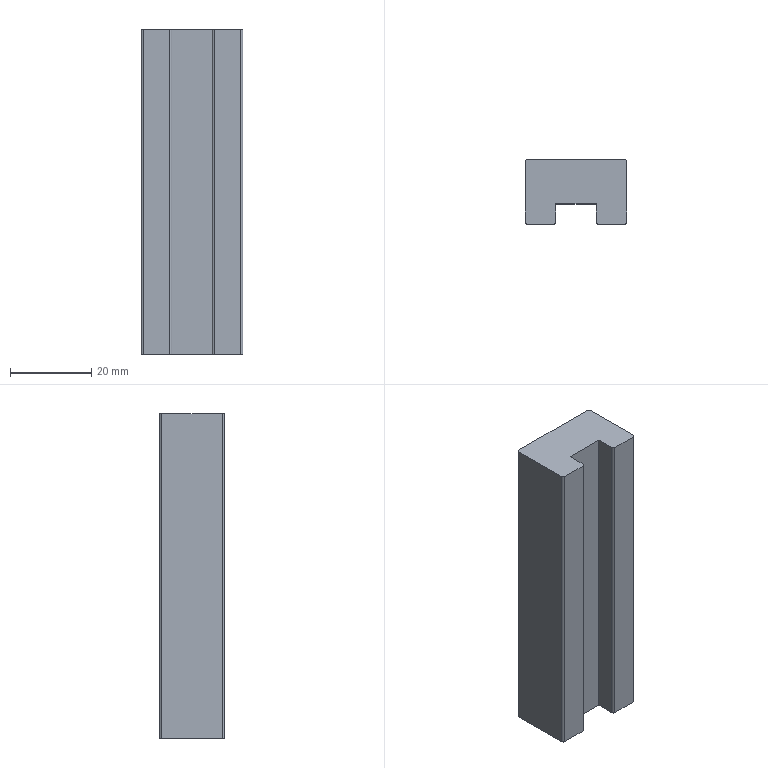Part | STEP file | 1 solid | 19 faces | box 25 x 16 x 80 mm | volume 27687 mm3 | plane 10 | cylinder 7 | cone 2 | commonest cylinder face diameters 1 x6 4.2 x1
STEP:
#1=CARTESIAN_POINT('',(0.,0.,0.));
#2=DIRECTION('',(0.,0.,1.));
#3=DIRECTION('',(1.,0.,0.));
#4=AXIS2_PLACEMENT_3D('',#1,#2,#3);
#5=CARTESIAN_POINT('',(1189.747,499.155,-36.381));
#6=VERTEX_POINT('',#5);
#7=CARTESIAN_POINT('',(1187.247,499.155,-36.381));
#8=DIRECTION('',(0.,0.,1.));
#9=DIRECTION('',(1.,0.,0.));
#10=AXIS2_PLACEMENT_3D('',#7,#8,#9);
#11=CIRCLE('',#10,2.5);
#12=CARTESIAN_POINT('',(1175.247,491.155,-36.381));
#13=DIRECTION('',(0.,0.,1.));
#14=DIRECTION('',(-1.,0.,0.));
#15=AXIS2_PLACEMENT_3D('',#12,#13,#14);
#16=PLANE('',#15);
#17=CARTESIAN_POINT('',(-12.,-8.));
#18=DIRECTION('',(-1.,0.));
#19=AXIS2_PLACEMENT_2D('',#17,#18);
#20=CIRCLE('',#19,2.5);
#21=(GEOMETRIC_REPRESENTATION_CONTEXT(2)PARAMETRIC_REPRESENTATION_CONTEXT()REPRESENTATION_CONTEXT('',''));
#22=DEFINITIONAL_REPRESENTATION('',(#20),#21);
#23=PCURVE('',#16,#22);
#24=CARTESIAN_POINT('',(1187.247,499.155,-36.381));
#25=DIRECTION('',(0.,0.,-1.));
#26=DIRECTION('',(-1.,0.,0.));
#27=AXIS2_PLACEMENT_3D('',#24,#25,#26);
#28=CONICAL_SURFACE('',#27,2.5,0.7854);
#29=CARTESIAN_POINT('',(9.425,0.));
#30=DIRECTION('',(-1.,0.));
#31=VECTOR('',#30,1.);
#32=LINE('',#29,#31);
#33=(GEOMETRIC_REPRESENTATION_CONTEXT(2)PARAMETRIC_REPRESENTATION_CONTEXT()REPRESENTATION_CONTEXT('',''));
#34=DEFINITIONAL_REPRESENTATION('',(#32),#33);
#35=PCURVE('',#28,#34);
#36=SURFACE_CURVE('',#11,(#23,#35),.PCURVE_S1.);
#37=EDGE_CURVE('',#6,#6,#36,.T.);
#38=ORIENTED_EDGE('',*,*,#37,.T.);
#39=EDGE_LOOP('',(#38));
#40=FACE_BOUND('',#39,.T.);
#41=CARTESIAN_POINT('',(1174.747,506.155,-36.381));
#42=VERTEX_POINT('',#41);
#43=CARTESIAN_POINT('',(1174.747,491.155,-36.381));
#44=VERTEX_POINT('',#43);
#45=CARTESIAN_POINT('',(1174.747,506.155,-36.381));
#46=DIRECTION('',(0.,-1.,0.));
#47=VECTOR('',#46,1.);
#48=LINE('',#45,#47);
#49=CARTESIAN_POINT('',(0.5,-15.));
#50=DIRECTION('',(0.,1.));
#51=VECTOR('',#50,1.);
#52=LINE('',#49,#51);
#53=(GEOMETRIC_REPRESENTATION_CONTEXT(2)PARAMETRIC_REPRESENTATION_CONTEXT()REPRESENTATION_CONTEXT('',''));
#54=DEFINITIONAL_REPRESENTATION('',(#52),#53);
#55=PCURVE('',#16,#54);
#56=CARTESIAN_POINT('',(1174.747,506.155,-36.381));
#57=DIRECTION('',(-1.,0.,0.));
#58=DIRECTION('',(0.,0.,-1.));
#59=AXIS2_PLACEMENT_3D('',#56,#57,#58);
#60=PLANE('',#59);
#61=CARTESIAN_POINT('',(0.,0.));
#62=DIRECTION('',(0.,1.));
#63=VECTOR('',#62,1.);
#64=LINE('',#61,#63);
#65=(GEOMETRIC_REPRESENTATION_CONTEXT(2)PARAMETRIC_REPRESENTATION_CONTEXT()REPRESENTATION_CONTEXT('',''));
#66=DEFINITIONAL_REPRESENTATION('',(#64),#65);
#67=PCURVE('',#60,#66);
#68=SURFACE_CURVE('',#48,(#55,#67),.PCURVE_S1.);
#69=EDGE_CURVE('',#42,#44,#68,.T.);
#70=ORIENTED_EDGE('',*,*,#69,.F.);
#71=CARTESIAN_POINT('',(1175.247,506.655,-36.381));
#72=VERTEX_POINT('',#71);
#73=CARTESIAN_POINT('',(1175.247,506.155,-36.381));
#74=DIRECTION('',(0.,0.,1.));
#75=DIRECTION('',(-1.,0.,0.));
#76=AXIS2_PLACEMENT_3D('',#73,#74,#75);
#77=CIRCLE('',#76,0.5);
#78=CARTESIAN_POINT('',(0.,-15.));
#79=DIRECTION('',(1.,0.));
#80=AXIS2_PLACEMENT_2D('',#78,#79);
#81=CIRCLE('',#80,0.5);
#82=(GEOMETRIC_REPRESENTATION_CONTEXT(2)PARAMETRIC_REPRESENTATION_CONTEXT()REPRESENTATION_CONTEXT('',''));
#83=DEFINITIONAL_REPRESENTATION('',(#81),#82);
#84=PCURVE('',#16,#83);
#85=CARTESIAN_POINT('',(1175.247,506.155,-36.381));
#86=DIRECTION('',(0.,0.,1.));
#87=DIRECTION('',(-1.,0.,0.));
#88=AXIS2_PLACEMENT_3D('',#85,#86,#87);
#89=CYLINDRICAL_SURFACE('',#88,0.5);
#90=CARTESIAN_POINT('',(0.,0.));
#91=DIRECTION('',(1.,0.));
#92=VECTOR('',#91,1.);
#93=LINE('',#90,#92);
#94=(GEOMETRIC_REPRESENTATION_CONTEXT(2)PARAMETRIC_REPRESENTATION_CONTEXT()REPRESENTATION_CONTEXT('',''));
#95=DEFINITIONAL_REPRESENTATION('',(#93),#94);
#96=PCURVE('',#89,#95);
#97=SURFACE_CURVE('',#77,(#84,#96),.PCURVE_S1.);
#98=EDGE_CURVE('',#72,#42,#97,.T.);
#99=ORIENTED_EDGE('',*,*,#98,.F.);
#100=CARTESIAN_POINT('',(1199.247,506.655,-36.381));
#101=VERTEX_POINT('',#100);
#102=CARTESIAN_POINT('',(1199.247,506.655,-36.381));
#103=DIRECTION('',(-1.,0.,0.));
#104=VECTOR('',#103,1.);
#105=LINE('',#102,#104);
#106=CARTESIAN_POINT('',(-24.,-15.5));
#107=DIRECTION('',(1.,0.));
#108=VECTOR('',#107,1.);
#109=LINE('',#106,#108);
#110=(GEOMETRIC_REPRESENTATION_CONTEXT(2)PARAMETRIC_REPRESENTATION_CONTEXT()REPRESENTATION_CONTEXT('',''));
#111=DEFINITIONAL_REPRESENTATION('',(#109),#110);
#112=PCURVE('',#16,#111);
#113=CARTESIAN_POINT('',(1199.247,506.655,-36.381));
#114=DIRECTION('',(0.,1.,0.));
#115=DIRECTION('',(0.,0.,1.));
#116=AXIS2_PLACEMENT_3D('',#113,#114,#115);
#117=PLANE('',#116);
#118=CARTESIAN_POINT('',(0.,0.));
#119=DIRECTION('',(0.,-1.));
#120=VECTOR('',#119,1.);
#121=LINE('',#118,#120);
#122=(GEOMETRIC_REPRESENTATION_CONTEXT(2)PARAMETRIC_REPRESENTATION_CONTEXT()REPRESENTATION_CONTEXT('',''));
#123=DEFINITIONAL_REPRESENTATION('',(#121),#122);
#124=PCURVE('',#117,#123);
#125=SURFACE_CURVE('',#105,(#112,#124),.PCURVE_S1.);
#126=EDGE_CURVE('',#101,#72,#125,.T.);
#127=ORIENTED_EDGE('',*,*,#126,.F.);
#128=CARTESIAN_POINT('',(1199.747,506.155,-36.381));
#129=VERTEX_POINT('',#128);
#130=CARTESIAN_POINT('',(1199.247,506.155,-36.381));
#131=DIRECTION('',(0.,0.,1.));
#132=DIRECTION('',(-1.,0.,0.));
#133=AXIS2_PLACEMENT_3D('',#130,#131,#132);
#134=CIRCLE('',#133,0.5);
#135=CARTESIAN_POINT('',(-24.,-15.));
#136=DIRECTION('',(1.,0.));
#137=AXIS2_PLACEMENT_2D('',#135,#136);
#138=CIRCLE('',#137,0.5);
#139=(GEOMETRIC_REPRESENTATION_CONTEXT(2)PARAMETRIC_REPRESENTATION_CONTEXT()REPRESENTATION_CONTEXT('',''));
#140=DEFINITIONAL_REPRESENTATION('',(#138),#139);
#141=PCURVE('',#16,#140);
#142=CARTESIAN_POINT('',(1199.247,506.155,-36.381));
#143=DIRECTION('',(0.,0.,1.));
#144=DIRECTION('',(-1.,0.,0.));
#145=AXIS2_PLACEMENT_3D('',#142,#143,#144);
#146=CYLINDRICAL_SURFACE('',#145,0.5);
#147=CARTESIAN_POINT('',(0.,0.));
#148=DIRECTION('',(1.,0.));
#149=VECTOR('',#148,1.);
#150=LINE('',#147,#149);
#151=(GEOMETRIC_REPRESENTATION_CONTEXT(2)PARAMETRIC_REPRESENTATION_CONTEXT()REPRESENTATION_CONTEXT('',''));
#152=DEFINITIONAL_REPRESENTATION('',(#150),#151);
#153=PCURVE('',#146,#152);
#154=SURFACE_CURVE('',#134,(#141,#153),.PCURVE_S1.);
#155=EDGE_CURVE('',#129,#101,#154,.T.);
#156=ORIENTED_EDGE('',*,*,#155,.F.);
#157=CARTESIAN_POINT('',(1199.747,491.155,-36.381));
#158=VERTEX_POINT('',#157);
#159=CARTESIAN_POINT('',(1199.747,491.155,-36.381));
#160=DIRECTION('',(0.,1.,0.));
#161=VECTOR('',#160,1.);
#162=LINE('',#159,#161);
#163=CARTESIAN_POINT('',(-24.5,0.));
#164=DIRECTION('',(0.,-1.));
#165=VECTOR('',#164,1.);
#166=LINE('',#163,#165);
#167=(GEOMETRIC_REPRESENTATION_CONTEXT(2)PARAMETRIC_REPRESENTATION_CONTEXT()REPRESENTATION_CONTEXT('',''));
#168=DEFINITIONAL_REPRESENTATION('',(#166),#167);
#169=PCURVE('',#16,#168);
#170=CARTESIAN_POINT('',(1199.747,491.155,-36.381));
#171=DIRECTION('',(1.,0.,0.));
#172=DIRECTION('',(0.,0.,1.));
#173=AXIS2_PLACEMENT_3D('',#170,#171,#172);
#174=PLANE('',#173);
#175=CARTESIAN_POINT('',(0.,0.));
#176=DIRECTION('',(0.,-1.));
#177=VECTOR('',#176,1.);
#178=LINE('',#175,#177);
#179=(GEOMETRIC_REPRESENTATION_CONTEXT(2)PARAMETRIC_REPRESENTATION_CONTEXT()REPRESENTATION_CONTEXT('',''));
#180=DEFINITIONAL_REPRESENTATION('',(#178),#179);
#181=PCURVE('',#174,#180);
#182=SURFACE_CURVE('',#162,(#169,#181),.PCURVE_S1.);
#183=EDGE_CURVE('',#158,#129,#182,.T.);
#184=ORIENTED_EDGE('',*,*,#183,.F.);
#185=CARTESIAN_POINT('',(1199.247,490.655,-36.381));
#186=VERTEX_POINT('',#185);
#187=CARTESIAN_POINT('',(1199.247,491.155,-36.381));
#188=DIRECTION('',(0.,0.,1.));
#189=DIRECTION('',(-1.,0.,0.));
#190=AXIS2_PLACEMENT_3D('',#187,#188,#189);
#191=CIRCLE('',#190,0.5);
#192=CARTESIAN_POINT('',(-24.,0.));
#193=DIRECTION('',(1.,0.));
#194=AXIS2_PLACEMENT_2D('',#192,#193);
#195=CIRCLE('',#194,0.5);
#196=(GEOMETRIC_REPRESENTATION_CONTEXT(2)PARAMETRIC_REPRESENTATION_CONTEXT()REPRESENTATION_CONTEXT('',''));
#197=DEFINITIONAL_REPRESENTATION('',(#195),#196);
#198=PCURVE('',#16,#197);
#199=CARTESIAN_POINT('',(1199.247,491.155,-36.381));
#200=DIRECTION('',(0.,0.,1.));
#201=DIRECTION('',(-1.,0.,0.));
#202=AXIS2_PLACEMENT_3D('',#199,#200,#201);
#203=CYLINDRICAL_SURFACE('',#202,0.5);
#204=CARTESIAN_POINT('',(0.,0.));
#205=DIRECTION('',(1.,0.));
#206=VECTOR('',#205,1.);
#207=LINE('',#204,#206);
#208=(GEOMETRIC_REPRESENTATION_CONTEXT(2)PARAMETRIC_REPRESENTATION_CONTEXT()REPRESENTATION_CONTEXT('',''));
#209=DEFINITIONAL_REPRESENTATION('',(#207),#208);
#210=PCURVE('',#203,#209);
#211=SURFACE_CURVE('',#191,(#198,#210),.PCURVE_S1.);
#212=EDGE_CURVE('',#186,#158,#211,.T.);
#213=ORIENTED_EDGE('',*,*,#212,.F.);
#214=CARTESIAN_POINT('',(1192.747,490.655,-36.381));
#215=VERTEX_POINT('',#214);
#216=CARTESIAN_POINT('',(1192.747,490.655,-36.381));
#217=DIRECTION('',(1.,0.,0.));
#218=VECTOR('',#217,1.);
#219=LINE('',#216,#218);
#220=CARTESIAN_POINT('',(-17.5,0.5));
#221=DIRECTION('',(-1.,0.));
#222=VECTOR('',#221,1.);
#223=LINE('',#220,#222);
#224=(GEOMETRIC_REPRESENTATION_CONTEXT(2)PARAMETRIC_REPRESENTATION_CONTEXT()REPRESENTATION_CONTEXT('',''));
#225=DEFINITIONAL_REPRESENTATION('',(#223),#224);
#226=PCURVE('',#16,#225);
#227=CARTESIAN_POINT('',(1192.747,490.655,-36.381));
#228=DIRECTION('',(0.,-1.,0.));
#229=DIRECTION('',(0.,0.,-1.));
#230=AXIS2_PLACEMENT_3D('',#227,#228,#229);
#231=PLANE('',#230);
#232=CARTESIAN_POINT('',(0.,0.));
#233=DIRECTION('',(0.,1.));
#234=VECTOR('',#233,1.);
#235=LINE('',#232,#234);
#236=(GEOMETRIC_REPRESENTATION_CONTEXT(2)PARAMETRIC_REPRESENTATION_CONTEXT()REPRESENTATION_CONTEXT('',''));
#237=DEFINITIONAL_REPRESENTATION('',(#235),#236);
#238=PCURVE('',#231,#237);
#239=SURFACE_CURVE('',#219,(#226,#238),.PCURVE_S1.);
#240=EDGE_CURVE('',#215,#186,#239,.T.);
#241=ORIENTED_EDGE('',*,*,#240,.F.);
#242=CARTESIAN_POINT('',(1192.247,491.155,-36.381));
#243=VERTEX_POINT('',#242);
#244=CARTESIAN_POINT('',(1192.747,491.155,-36.381));
#245=DIRECTION('',(0.,0.,1.));
#246=DIRECTION('',(-1.,0.,0.));
#247=AXIS2_PLACEMENT_3D('',#244,#245,#246);
#248=CIRCLE('',#247,0.5);
#249=CARTESIAN_POINT('',(-17.5,0.));
#250=DIRECTION('',(1.,0.));
#251=AXIS2_PLACEMENT_2D('',#249,#250);
#252=CIRCLE('',#251,0.5);
#253=(GEOMETRIC_REPRESENTATION_CONTEXT(2)PARAMETRIC_REPRESENTATION_CONTEXT()REPRESENTATION_CONTEXT('',''));
#254=DEFINITIONAL_REPRESENTATION('',(#252),#253);
#255=PCURVE('',#16,#254);
#256=CARTESIAN_POINT('',(1192.747,491.155,-36.381));
#257=DIRECTION('',(0.,0.,1.));
#258=DIRECTION('',(-1.,0.,0.));
#259=AXIS2_PLACEMENT_3D('',#256,#257,#258);
#260=CYLINDRICAL_SURFACE('',#259,0.5);
#261=CARTESIAN_POINT('',(0.,0.));
#262=DIRECTION('',(1.,0.));
#263=VECTOR('',#262,1.);
#264=LINE('',#261,#263);
#265=(GEOMETRIC_REPRESENTATION_CONTEXT(2)PARAMETRIC_REPRESENTATION_CONTEXT()REPRESENTATION_CONTEXT('',''));
#266=DEFINITIONAL_REPRESENTATION('',(#264),#265);
#267=PCURVE('',#260,#266);
#268=SURFACE_CURVE('',#248,(#255,#267),.PCURVE_S1.);
#269=EDGE_CURVE('',#243,#215,#268,.T.);
#270=ORIENTED_EDGE('',*,*,#269,.F.);
#271=CARTESIAN_POINT('',(1192.247,495.655,-36.381));
#272=VERTEX_POINT('',#271);
#273=CARTESIAN_POINT('',(1192.247,495.655,-36.381));
#274=DIRECTION('',(0.,-1.,0.));
#275=VECTOR('',#274,1.);
#276=LINE('',#273,#275);
#277=CARTESIAN_POINT('',(-17.,-4.5));
#278=DIRECTION('',(0.,1.));
#279=VECTOR('',#278,1.);
#280=LINE('',#277,#279);
#281=(GEOMETRIC_REPRESENTATION_CONTEXT(2)PARAMETRIC_REPRESENTATION_CONTEXT()REPRESENTATION_CONTEXT('',''));
#282=DEFINITIONAL_REPRESENTATION('',(#280),#281);
#283=PCURVE('',#16,#282);
#284=CARTESIAN_POINT('',(1192.247,495.655,-36.381));
#285=DIRECTION('',(-1.,0.,0.));
#286=DIRECTION('',(0.,0.,-1.));
#287=AXIS2_PLACEMENT_3D('',#284,#285,#286);
#288=PLANE('',#287);
#289=CARTESIAN_POINT('',(0.,0.));
#290=DIRECTION('',(0.,1.));
#291=VECTOR('',#290,1.);
#292=LINE('',#289,#291);
#293=(GEOMETRIC_REPRESENTATION_CONTEXT(2)PARAMETRIC_REPRESENTATION_CONTEXT()REPRESENTATION_CONTEXT('',''));
#294=DEFINITIONAL_REPRESENTATION('',(#292),#293);
#295=PCURVE('',#288,#294);
#296=SURFACE_CURVE('',#276,(#283,#295),.PCURVE_S1.);
#297=EDGE_CURVE('',#272,#243,#296,.T.);
#298=ORIENTED_EDGE('',*,*,#297,.F.);
#299=CARTESIAN_POINT('',(1182.247,495.655,-36.381));
#300=VERTEX_POINT('',#299);
#301=CARTESIAN_POINT('',(1182.247,495.655,-36.381));
#302=DIRECTION('',(1.,0.,0.));
#303=VECTOR('',#302,1.);
#304=LINE('',#301,#303);
#305=CARTESIAN_POINT('',(-7.,-4.5));
#306=DIRECTION('',(-1.,0.));
#307=VECTOR('',#306,1.);
#308=LINE('',#305,#307);
#309=(GEOMETRIC_REPRESENTATION_CONTEXT(2)PARAMETRIC_REPRESENTATION_CONTEXT()REPRESENTATION_CONTEXT('',''));
#310=DEFINITIONAL_REPRESENTATION('',(#308),#309);
#311=PCURVE('',#16,#310);
#312=CARTESIAN_POINT('',(1182.247,495.655,-36.381));
#313=DIRECTION('',(0.,-1.,0.));
#314=DIRECTION('',(0.,0.,-1.));
#315=AXIS2_PLACEMENT_3D('',#312,#313,#314);
#316=PLANE('',#315);
#317=CARTESIAN_POINT('',(0.,0.));
#318=DIRECTION('',(0.,1.));
#319=VECTOR('',#318,1.);
#320=LINE('',#317,#319);
#321=(GEOMETRIC_REPRESENTATION_CONTEXT(2)PARAMETRIC_REPRESENTATION_CONTEXT()REPRESENTATION_CONTEXT('',''));
#322=DEFINITIONAL_REPRESENTATION('',(#320),#321);
#323=PCURVE('',#316,#322);
#324=SURFACE_CURVE('',#304,(#311,#323),.PCURVE_S1.);
#325=EDGE_CURVE('',#300,#272,#324,.T.);
#326=ORIENTED_EDGE('',*,*,#325,.F.);
#327=CARTESIAN_POINT('',(1182.247,491.155,-36.381));
#328=VERTEX_POINT('',#327);
#329=CARTESIAN_POINT('',(1182.247,491.155,-36.381));
#330=DIRECTION('',(0.,1.,0.));
#331=VECTOR('',#330,1.);
#332=LINE('',#329,#331);
#333=CARTESIAN_POINT('',(-7.,0.));
#334=DIRECTION('',(0.,-1.));
#335=VECTOR('',#334,1.);
#336=LINE('',#333,#335);
#337=(GEOMETRIC_REPRESENTATION_CONTEXT(2)PARAMETRIC_REPRESENTATION_CONTEXT()REPRESENTATION_CONTEXT('',''));
#338=DEFINITIONAL_REPRESENTATION('',(#336),#337);
#339=PCURVE('',#16,#338);
#340=CARTESIAN_POINT('',(1182.247,491.155,-36.381));
#341=DIRECTION('',(1.,0.,0.));
#342=DIRECTION('',(0.,0.,1.));
#343=AXIS2_PLACEMENT_3D('',#340,#341,#342);
#344=PLANE('',#343);
#345=CARTESIAN_POINT('',(0.,0.));
#346=DIRECTION('',(0.,-1.));
#347=VECTOR('',#346,1.);
#348=LINE('',#345,#347);
#349=(GEOMETRIC_REPRESENTATION_CONTEXT(2)PARAMETRIC_REPRESENTATION_CONTEXT()REPRESENTATION_CONTEXT('',''));
#350=DEFINITIONAL_REPRESENTATION('',(#348),#349);
#351=PCURVE('',#344,#350);
#352=SURFACE_CURVE('',#332,(#339,#351),.PCURVE_S1.);
#353=EDGE_CURVE('',#328,#300,#352,.T.);
#354=ORIENTED_EDGE('',*,*,#353,.F.);
#355=CARTESIAN_POINT('',(1181.747,490.655,-36.381));
#356=VERTEX_POINT('',#355);
#357=CARTESIAN_POINT('',(1181.747,491.155,-36.381));
#358=DIRECTION('',(0.,0.,1.));
#359=DIRECTION('',(-1.,0.,0.));
#360=AXIS2_PLACEMENT_3D('',#357,#358,#359);
#361=CIRCLE('',#360,0.5);
#362=CARTESIAN_POINT('',(-6.5,0.));
#363=DIRECTION('',(1.,0.));
#364=AXIS2_PLACEMENT_2D('',#362,#363);
#365=CIRCLE('',#364,0.5);
#366=(GEOMETRIC_REPRESENTATION_CONTEXT(2)PARAMETRIC_REPRESENTATION_CONTEXT()REPRESENTATION_CONTEXT('',''));
#367=DEFINITIONAL_REPRESENTATION('',(#365),#366);
#368=PCURVE('',#16,#367);
#369=CARTESIAN_POINT('',(1181.747,491.155,-36.381));
#370=DIRECTION('',(0.,0.,1.));
#371=DIRECTION('',(-1.,0.,0.));
#372=AXIS2_PLACEMENT_3D('',#369,#370,#371);
#373=CYLINDRICAL_SURFACE('',#372,0.5);
#374=CARTESIAN_POINT('',(0.,0.));
#375=DIRECTION('',(1.,0.));
#376=VECTOR('',#375,1.);
#377=LINE('',#374,#376);
#378=(GEOMETRIC_REPRESENTATION_CONTEXT(2)PARAMETRIC_REPRESENTATION_CONTEXT()REPRESENTATION_CONTEXT('',''));
#379=DEFINITIONAL_REPRESENTATION('',(#377),#378);
#380=PCURVE('',#373,#379);
#381=SURFACE_CURVE('',#361,(#368,#380),.PCURVE_S1.);
#382=EDGE_CURVE('',#356,#328,#381,.T.);
#383=ORIENTED_EDGE('',*,*,#382,.F.);
#384=CARTESIAN_POINT('',(1175.247,490.655,-36.381));
#385=VERTEX_POINT('',#384);
#386=CARTESIAN_POINT('',(1175.247,490.655,-36.381));
#387=DIRECTION('',(1.,0.,0.));
#388=VECTOR('',#387,1.);
#389=LINE('',#386,#388);
#390=CARTESIAN_POINT('',(0.,0.5));
#391=DIRECTION('',(-1.,0.));
#392=VECTOR('',#391,1.);
#393=LINE('',#390,#392);
#394=(GEOMETRIC_REPRESENTATION_CONTEXT(2)PARAMETRIC_REPRESENTATION_CONTEXT()REPRESENTATION_CONTEXT('',''));
#395=DEFINITIONAL_REPRESENTATION('',(#393),#394);
#396=PCURVE('',#16,#395);
#397=CARTESIAN_POINT('',(1175.247,490.655,-36.381));
#398=DIRECTION('',(0.,-1.,0.));
#399=DIRECTION('',(0.,0.,-1.));
#400=AXIS2_PLACEMENT_3D('',#397,#398,#399);
#401=PLANE('',#400);
#402=CARTESIAN_POINT('',(0.,0.));
#403=DIRECTION('',(0.,1.));
#404=VECTOR('',#403,1.);
#405=LINE('',#402,#404);
#406=(GEOMETRIC_REPRESENTATION_CONTEXT(2)PARAMETRIC_REPRESENTATION_CONTEXT()REPRESENTATION_CONTEXT('',''));
#407=DEFINITIONAL_REPRESENTATION('',(#405),#406);
#408=PCURVE('',#401,#407);
#409=SURFACE_CURVE('',#389,(#396,#408),.PCURVE_S1.);
#410=EDGE_CURVE('',#385,#356,#409,.T.);
#411=ORIENTED_EDGE('',*,*,#410,.F.);
#412=CARTESIAN_POINT('',(1175.247,491.155,-36.381));
#413=DIRECTION('',(0.,0.,1.));
#414=DIRECTION('',(-1.,0.,0.));
#415=AXIS2_PLACEMENT_3D('',#412,#413,#414);
#416=CIRCLE('',#415,0.5);
#417=CARTESIAN_POINT('',(0.,0.));
#418=DIRECTION('',(1.,0.));
#419=AXIS2_PLACEMENT_2D('',#417,#418);
#420=CIRCLE('',#419,0.5);
#421=(GEOMETRIC_REPRESENTATION_CONTEXT(2)PARAMETRIC_REPRESENTATION_CONTEXT()REPRESENTATION_CONTEXT('',''));
#422=DEFINITIONAL_REPRESENTATION('',(#420),#421);
#423=PCURVE('',#16,#422);
#424=CARTESIAN_POINT('',(1175.247,491.155,-36.381));
#425=DIRECTION('',(0.,0.,1.));
#426=DIRECTION('',(-1.,0.,0.));
#427=AXIS2_PLACEMENT_3D('',#424,#425,#426);
#428=CYLINDRICAL_SURFACE('',#427,0.5);
#429=CARTESIAN_POINT('',(0.,0.));
#430=DIRECTION('',(1.,0.));
#431=VECTOR('',#430,1.);
#432=LINE('',#429,#431);
#433=(GEOMETRIC_REPRESENTATION_CONTEXT(2)PARAMETRIC_REPRESENTATION_CONTEXT()REPRESENTATION_CONTEXT('',''));
#434=DEFINITIONAL_REPRESENTATION('',(#432),#433);
#435=PCURVE('',#428,#434);
#436=SURFACE_CURVE('',#416,(#423,#435),.PCURVE_S1.);
#437=EDGE_CURVE('',#44,#385,#436,.T.);
#438=ORIENTED_EDGE('',*,*,#437,.F.);
#439=EDGE_LOOP('',(#70,#99,#127,#156,#184,#213,#241,#270,#298,#326,#354,#383,#411,#438));
#440=FACE_BOUND('',#439,.T.);
#441=ADVANCED_FACE('',(#40,#440),#16,.F.);
#442=CARTESIAN_POINT('',(1174.747,506.155,43.619));
#443=VERTEX_POINT('',#442);
#444=CARTESIAN_POINT('',(1174.747,491.155,43.619));
#445=VERTEX_POINT('',#444);
#446=CARTESIAN_POINT('',(1174.747,506.155,43.619));
#447=DIRECTION('',(0.,-1.,0.));
#448=VECTOR('',#447,1.);
#449=LINE('',#446,#448);
#450=CARTESIAN_POINT('',(-80.,0.));
#451=DIRECTION('',(0.,1.));
#452=VECTOR('',#451,1.);
#453=LINE('',#450,#452);
#454=(GEOMETRIC_REPRESENTATION_CONTEXT(2)PARAMETRIC_REPRESENTATION_CONTEXT()REPRESENTATION_CONTEXT('',''));
#455=DEFINITIONAL_REPRESENTATION('',(#453),#454);
#456=PCURVE('',#60,#455);
#457=CARTESIAN_POINT('',(1175.247,491.155,43.619));
#458=DIRECTION('',(0.,0.,1.));
#459=DIRECTION('',(-1.,0.,0.));
#460=AXIS2_PLACEMENT_3D('',#457,#458,#459);
#461=PLANE('',#460);
#462=CARTESIAN_POINT('',(0.5,-15.));
#463=DIRECTION('',(0.,1.));
#464=VECTOR('',#463,1.);
#465=LINE('',#462,#464);
#466=(GEOMETRIC_REPRESENTATION_CONTEXT(2)PARAMETRIC_REPRESENTATION_CONTEXT()REPRESENTATION_CONTEXT('',''));
#467=DEFINITIONAL_REPRESENTATION('',(#465),#466);
#468=PCURVE('',#461,#467);
#469=SURFACE_CURVE('',#449,(#456,#468),.PCURVE_S1.);
#470=EDGE_CURVE('',#443,#445,#469,.T.);
#471=ORIENTED_EDGE('',*,*,#470,.F.);
#472=CARTESIAN_POINT('',(1174.747,506.155,-36.381));
#473=DIRECTION('',(0.,0.,1.));
#474=VECTOR('',#473,1.);
#475=LINE('',#472,#474);
#476=CARTESIAN_POINT('',(0.,0.));
#477=DIRECTION('',(-1.,0.));
#478=VECTOR('',#477,1.);
#479=LINE('',#476,#478);
#480=(GEOMETRIC_REPRESENTATION_CONTEXT(2)PARAMETRIC_REPRESENTATION_CONTEXT()REPRESENTATION_CONTEXT('',''));
#481=DEFINITIONAL_REPRESENTATION('',(#479),#480);
#482=PCURVE('',#60,#481);
#483=CARTESIAN_POINT('',(6.283,0.));
#484=DIRECTION('',(0.,1.));
#485=VECTOR('',#484,1.);
#486=LINE('',#483,#485);
#487=(GEOMETRIC_REPRESENTATION_CONTEXT(2)PARAMETRIC_REPRESENTATION_CONTEXT()REPRESENTATION_CONTEXT('',''));
#488=DEFINITIONAL_REPRESENTATION('',(#486),#487);
#489=PCURVE('',#89,#488);
#490=SURFACE_CURVE('',#475,(#482,#489),.PCURVE_S1.);
#491=EDGE_CURVE('',#42,#443,#490,.T.);
#492=ORIENTED_EDGE('',*,*,#491,.F.);
#493=ORIENTED_EDGE('',*,*,#69,.T.);
#494=CARTESIAN_POINT('',(1174.747,491.155,-36.381));
#495=DIRECTION('',(0.,0.,1.));
#496=VECTOR('',#495,1.);
#497=LINE('',#494,#496);
#498=CARTESIAN_POINT('',(0.,15.));
#499=DIRECTION('',(-1.,0.));
#500=VECTOR('',#499,1.);
#501=LINE('',#498,#500);
#502=(GEOMETRIC_REPRESENTATION_CONTEXT(2)PARAMETRIC_REPRESENTATION_CONTEXT()REPRESENTATION_CONTEXT('',''));
#503=DEFINITIONAL_REPRESENTATION('',(#501),#502);
#504=PCURVE('',#60,#503);
#505=CARTESIAN_POINT('',(0.,0.));
#506=DIRECTION('',(0.,1.));
#507=VECTOR('',#506,1.);
#508=LINE('',#505,#507);
#509=(GEOMETRIC_REPRESENTATION_CONTEXT(2)PARAMETRIC_REPRESENTATION_CONTEXT()REPRESENTATION_CONTEXT('',''));
#510=DEFINITIONAL_REPRESENTATION('',(#508),#509);
#511=PCURVE('',#428,#510);
#512=SURFACE_CURVE('',#497,(#504,#511),.PCURVE_S1.);
#513=EDGE_CURVE('',#44,#445,#512,.T.);
#514=ORIENTED_EDGE('',*,*,#513,.T.);
#515=EDGE_LOOP('',(#471,#492,#493,#514));
#516=FACE_BOUND('',#515,.T.);
#517=ADVANCED_FACE('',(#516),#60,.T.);
#518=CARTESIAN_POINT('',(1175.247,490.655,43.619));
#519=VERTEX_POINT('',#518);
#520=CARTESIAN_POINT('',(1175.247,491.155,43.619));
#521=DIRECTION('',(0.,0.,1.));
#522=DIRECTION('',(-1.,0.,0.));
#523=AXIS2_PLACEMENT_3D('',#520,#521,#522);
#524=CIRCLE('',#523,0.5);
#525=CARTESIAN_POINT('',(0.,80.));
#526=DIRECTION('',(1.,0.));
#527=VECTOR('',#526,1.);
#528=LINE('',#525,#527);
#529=(GEOMETRIC_REPRESENTATION_CONTEXT(2)PARAMETRIC_REPRESENTATION_CONTEXT()REPRESENTATION_CONTEXT('',''));
#530=DEFINITIONAL_REPRESENTATION('',(#528),#529);
#531=PCURVE('',#428,#530);
#532=CARTESIAN_POINT('',(0.,0.));
#533=DIRECTION('',(1.,0.));
#534=AXIS2_PLACEMENT_2D('',#532,#533);
#535=CIRCLE('',#534,0.5);
#536=(GEOMETRIC_REPRESENTATION_CONTEXT(2)PARAMETRIC_REPRESENTATION_CONTEXT()REPRESENTATION_CONTEXT('',''));
#537=DEFINITIONAL_REPRESENTATION('',(#535),#536);
#538=PCURVE('',#461,#537);
#539=SURFACE_CURVE('',#524,(#531,#538),.PCURVE_S1.);
#540=EDGE_CURVE('',#445,#519,#539,.T.);
#541=ORIENTED_EDGE('',*,*,#540,.F.);
#542=ORIENTED_EDGE('',*,*,#513,.F.);
#543=ORIENTED_EDGE('',*,*,#437,.T.);
#544=CARTESIAN_POINT('',(1175.247,490.655,-36.381));
#545=DIRECTION('',(0.,0.,1.));
#546=VECTOR('',#545,1.);
#547=LINE('',#544,#546);
#548=CARTESIAN_POINT('',(1.571,0.));
#549=DIRECTION('',(0.,1.));
#550=VECTOR('',#549,1.);
#551=LINE('',#548,#550);
#552=(GEOMETRIC_REPRESENTATION_CONTEXT(2)PARAMETRIC_REPRESENTATION_CONTEXT()REPRESENTATION_CONTEXT('',''));
#553=DEFINITIONAL_REPRESENTATION('',(#551),#552);
#554=PCURVE('',#428,#553);
#555=CARTESIAN_POINT('',(0.,0.));
#556=DIRECTION('',(-1.,0.));
#557=VECTOR('',#556,1.);
#558=LINE('',#555,#557);
#559=(GEOMETRIC_REPRESENTATION_CONTEXT(2)PARAMETRIC_REPRESENTATION_CONTEXT()REPRESENTATION_CONTEXT('',''));
#560=DEFINITIONAL_REPRESENTATION('',(#558),#559);
#561=PCURVE('',#401,#560);
#562=SURFACE_CURVE('',#547,(#554,#561),.PCURVE_S1.);
#563=EDGE_CURVE('',#385,#519,#562,.T.);
#564=ORIENTED_EDGE('',*,*,#563,.T.);
#565=EDGE_LOOP('',(#541,#542,#543,#564));
#566=FACE_BOUND('',#565,.T.);
#567=ADVANCED_FACE('',(#566),#428,.T.);
#568=CARTESIAN_POINT('',(1181.747,490.655,43.619));
#569=VERTEX_POINT('',#568);
#570=CARTESIAN_POINT('',(1175.247,490.655,43.619));
#571=DIRECTION('',(1.,0.,0.));
#572=VECTOR('',#571,1.);
#573=LINE('',#570,#572);
#574=CARTESIAN_POINT('',(-80.,0.));
#575=DIRECTION('',(0.,1.));
#576=VECTOR('',#575,1.);
#577=LINE('',#574,#576);
#578=(GEOMETRIC_REPRESENTATION_CONTEXT(2)PARAMETRIC_REPRESENTATION_CONTEXT()REPRESENTATION_CONTEXT('',''));
#579=DEFINITIONAL_REPRESENTATION('',(#577),#578);
#580=PCURVE('',#401,#579);
#581=CARTESIAN_POINT('',(0.,0.5));
#582=DIRECTION('',(-1.,0.));
#583=VECTOR('',#582,1.);
#584=LINE('',#581,#583);
#585=(GEOMETRIC_REPRESENTATION_CONTEXT(2)PARAMETRIC_REPRESENTATION_CONTEXT()REPRESENTATION_CONTEXT('',''));
#586=DEFINITIONAL_REPRESENTATION('',(#584),#585);
#587=PCURVE('',#461,#586);
#588=SURFACE_CURVE('',#573,(#580,#587),.PCURVE_S1.);
#589=EDGE_CURVE('',#519,#569,#588,.T.);
#590=ORIENTED_EDGE('',*,*,#589,.F.);
#591=ORIENTED_EDGE('',*,*,#563,.F.);
#592=ORIENTED_EDGE('',*,*,#410,.T.);
#593=CARTESIAN_POINT('',(1181.747,490.655,-36.381));
#594=DIRECTION('',(0.,0.,1.));
#595=VECTOR('',#594,1.);
#596=LINE('',#593,#595);
#597=CARTESIAN_POINT('',(0.,6.5));
#598=DIRECTION('',(-1.,0.));
#599=VECTOR('',#598,1.);
#600=LINE('',#597,#599);
#601=(GEOMETRIC_REPRESENTATION_CONTEXT(2)PARAMETRIC_REPRESENTATION_CONTEXT()REPRESENTATION_CONTEXT('',''));
#602=DEFINITIONAL_REPRESENTATION('',(#600),#601);
#603=PCURVE('',#401,#602);
#604=CARTESIAN_POINT('',(1.571,0.));
#605=DIRECTION('',(0.,1.));
#606=VECTOR('',#605,1.);
#607=LINE('',#604,#606);
#608=(GEOMETRIC_REPRESENTATION_CONTEXT(2)PARAMETRIC_REPRESENTATION_CONTEXT()REPRESENTATION_CONTEXT('',''));
#609=DEFINITIONAL_REPRESENTATION('',(#607),#608);
#610=PCURVE('',#373,#609);
#611=SURFACE_CURVE('',#596,(#603,#610),.PCURVE_S1.);
#612=EDGE_CURVE('',#356,#569,#611,.T.);
#613=ORIENTED_EDGE('',*,*,#612,.T.);
#614=EDGE_LOOP('',(#590,#591,#592,#613));
#615=FACE_BOUND('',#614,.T.);
#616=ADVANCED_FACE('',(#615),#401,.T.);
#617=CARTESIAN_POINT('',(1182.247,491.155,43.619));
#618=VERTEX_POINT('',#617);
#619=CARTESIAN_POINT('',(1181.747,491.155,43.619));
#620=DIRECTION('',(0.,0.,1.));
#621=DIRECTION('',(-1.,0.,0.));
#622=AXIS2_PLACEMENT_3D('',#619,#620,#621);
#623=CIRCLE('',#622,0.5);
#624=CARTESIAN_POINT('',(0.,80.));
#625=DIRECTION('',(1.,0.));
#626=VECTOR('',#625,1.);
#627=LINE('',#624,#626);
#628=(GEOMETRIC_REPRESENTATION_CONTEXT(2)PARAMETRIC_REPRESENTATION_CONTEXT()REPRESENTATION_CONTEXT('',''));
#629=DEFINITIONAL_REPRESENTATION('',(#627),#628);
#630=PCURVE('',#373,#629);
#631=CARTESIAN_POINT('',(-6.5,0.));
#632=DIRECTION('',(1.,0.));
#633=AXIS2_PLACEMENT_2D('',#631,#632);
#634=CIRCLE('',#633,0.5);
#635=(GEOMETRIC_REPRESENTATION_CONTEXT(2)PARAMETRIC_REPRESENTATION_CONTEXT()REPRESENTATION_CONTEXT('',''));
#636=DEFINITIONAL_REPRESENTATION('',(#634),#635);
#637=PCURVE('',#461,#636);
#638=SURFACE_CURVE('',#623,(#630,#637),.PCURVE_S1.);
#639=EDGE_CURVE('',#569,#618,#638,.T.);
#640=ORIENTED_EDGE('',*,*,#639,.F.);
#641=ORIENTED_EDGE('',*,*,#612,.F.);
#642=ORIENTED_EDGE('',*,*,#382,.T.);
#643=CARTESIAN_POINT('',(1182.247,491.155,-36.381));
#644=DIRECTION('',(0.,0.,1.));
#645=VECTOR('',#644,1.);
#646=LINE('',#643,#645);
#647=CARTESIAN_POINT('',(3.142,0.));
#648=DIRECTION('',(0.,1.));
#649=VECTOR('',#648,1.);
#650=LINE('',#647,#649);
#651=(GEOMETRIC_REPRESENTATION_CONTEXT(2)PARAMETRIC_REPRESENTATION_CONTEXT()REPRESENTATION_CONTEXT('',''));
#652=DEFINITIONAL_REPRESENTATION('',(#650),#651);
#653=PCURVE('',#373,#652);
#654=CARTESIAN_POINT('',(0.,0.));
#655=DIRECTION('',(1.,0.));
#656=VECTOR('',#655,1.);
#657=LINE('',#654,#656);
#658=(GEOMETRIC_REPRESENTATION_CONTEXT(2)PARAMETRIC_REPRESENTATION_CONTEXT()REPRESENTATION_CONTEXT('',''));
#659=DEFINITIONAL_REPRESENTATION('',(#657),#658);
#660=PCURVE('',#344,#659);
#661=SURFACE_CURVE('',#646,(#653,#660),.PCURVE_S1.);
#662=EDGE_CURVE('',#328,#618,#661,.T.);
#663=ORIENTED_EDGE('',*,*,#662,.T.);
#664=EDGE_LOOP('',(#640,#641,#642,#663));
#665=FACE_BOUND('',#664,.T.);
#666=ADVANCED_FACE('',(#665),#373,.T.);
#667=CARTESIAN_POINT('',(1182.247,495.655,43.619));
#668=VERTEX_POINT('',#667);
#669=CARTESIAN_POINT('',(1182.247,491.155,43.619));
#670=DIRECTION('',(0.,1.,0.));
#671=VECTOR('',#670,1.);
#672=LINE('',#669,#671);
#673=CARTESIAN_POINT('',(80.,0.));
#674=DIRECTION('',(0.,-1.));
#675=VECTOR('',#674,1.);
#676=LINE('',#673,#675);
#677=(GEOMETRIC_REPRESENTATION_CONTEXT(2)PARAMETRIC_REPRESENTATION_CONTEXT()REPRESENTATION_CONTEXT('',''));
#678=DEFINITIONAL_REPRESENTATION('',(#676),#677);
#679=PCURVE('',#344,#678);
#680=CARTESIAN_POINT('',(-7.,0.));
#681=DIRECTION('',(0.,-1.));
#682=VECTOR('',#681,1.);
#683=LINE('',#680,#682);
#684=(GEOMETRIC_REPRESENTATION_CONTEXT(2)PARAMETRIC_REPRESENTATION_CONTEXT()REPRESENTATION_CONTEXT('',''));
#685=DEFINITIONAL_REPRESENTATION('',(#683),#684);
#686=PCURVE('',#461,#685);
#687=SURFACE_CURVE('',#672,(#679,#686),.PCURVE_S1.);
#688=EDGE_CURVE('',#618,#668,#687,.T.);
#689=ORIENTED_EDGE('',*,*,#688,.F.);
#690=ORIENTED_EDGE('',*,*,#662,.F.);
#691=ORIENTED_EDGE('',*,*,#353,.T.);
#692=CARTESIAN_POINT('',(1182.247,495.655,-36.381));
#693=DIRECTION('',(0.,0.,1.));
#694=VECTOR('',#693,1.);
#695=LINE('',#692,#694);
#696=CARTESIAN_POINT('',(0.,-4.5));
#697=DIRECTION('',(1.,0.));
#698=VECTOR('',#697,1.);
#699=LINE('',#696,#698);
#700=(GEOMETRIC_REPRESENTATION_CONTEXT(2)PARAMETRIC_REPRESENTATION_CONTEXT()REPRESENTATION_CONTEXT('',''));
#701=DEFINITIONAL_REPRESENTATION('',(#699),#700);
#702=PCURVE('',#344,#701);
#703=CARTESIAN_POINT('',(0.,0.));
#704=DIRECTION('',(-1.,0.));
#705=VECTOR('',#704,1.);
#706=LINE('',#703,#705);
#707=(GEOMETRIC_REPRESENTATION_CONTEXT(2)PARAMETRIC_REPRESENTATION_CONTEXT()REPRESENTATION_CONTEXT('',''));
#708=DEFINITIONAL_REPRESENTATION('',(#706),#707);
#709=PCURVE('',#316,#708);
#710=SURFACE_CURVE('',#695,(#702,#709),.PCURVE_S1.);
#711=EDGE_CURVE('',#300,#668,#710,.T.);
#712=ORIENTED_EDGE('',*,*,#711,.T.);
#713=EDGE_LOOP('',(#689,#690,#691,#712));
#714=FACE_BOUND('',#713,.T.);
#715=ADVANCED_FACE('',(#714),#344,.T.);
#716=CARTESIAN_POINT('',(1192.247,495.655,43.619));
#717=VERTEX_POINT('',#716);
#718=CARTESIAN_POINT('',(1182.247,495.655,43.619));
#719=DIRECTION('',(1.,0.,0.));
#720=VECTOR('',#719,1.);
#721=LINE('',#718,#720);
#722=CARTESIAN_POINT('',(-80.,0.));
#723=DIRECTION('',(0.,1.));
#724=VECTOR('',#723,1.);
#725=LINE('',#722,#724);
#726=(GEOMETRIC_REPRESENTATION_CONTEXT(2)PARAMETRIC_REPRESENTATION_CONTEXT()REPRESENTATION_CONTEXT('',''));
#727=DEFINITIONAL_REPRESENTATION('',(#725),#726);
#728=PCURVE('',#316,#727);
#729=CARTESIAN_POINT('',(-7.,-4.5));
#730=DIRECTION('',(-1.,0.));
#731=VECTOR('',#730,1.);
#732=LINE('',#729,#731);
#733=(GEOMETRIC_REPRESENTATION_CONTEXT(2)PARAMETRIC_REPRESENTATION_CONTEXT()REPRESENTATION_CONTEXT('',''));
#734=DEFINITIONAL_REPRESENTATION('',(#732),#733);
#735=PCURVE('',#461,#734);
#736=SURFACE_CURVE('',#721,(#728,#735),.PCURVE_S1.);
#737=EDGE_CURVE('',#668,#717,#736,.T.);
#738=ORIENTED_EDGE('',*,*,#737,.F.);
#739=ORIENTED_EDGE('',*,*,#711,.F.);
#740=ORIENTED_EDGE('',*,*,#325,.T.);
#741=CARTESIAN_POINT('',(1192.247,495.655,-36.381));
#742=DIRECTION('',(0.,0.,1.));
#743=VECTOR('',#742,1.);
#744=LINE('',#741,#743);
#745=CARTESIAN_POINT('',(0.,10.));
#746=DIRECTION('',(-1.,0.));
#747=VECTOR('',#746,1.);
#748=LINE('',#745,#747);
#749=(GEOMETRIC_REPRESENTATION_CONTEXT(2)PARAMETRIC_REPRESENTATION_CONTEXT()REPRESENTATION_CONTEXT('',''));
#750=DEFINITIONAL_REPRESENTATION('',(#748),#749);
#751=PCURVE('',#316,#750);
#752=CARTESIAN_POINT('',(0.,0.));
#753=DIRECTION('',(-1.,0.));
#754=VECTOR('',#753,1.);
#755=LINE('',#752,#754);
#756=(GEOMETRIC_REPRESENTATION_CONTEXT(2)PARAMETRIC_REPRESENTATION_CONTEXT()REPRESENTATION_CONTEXT('',''));
#757=DEFINITIONAL_REPRESENTATION('',(#755),#756);
#758=PCURVE('',#288,#757);
#759=SURFACE_CURVE('',#744,(#751,#758),.PCURVE_S1.);
#760=EDGE_CURVE('',#272,#717,#759,.T.);
#761=ORIENTED_EDGE('',*,*,#760,.T.);
#762=EDGE_LOOP('',(#738,#739,#740,#761));
#763=FACE_BOUND('',#762,.T.);
#764=ADVANCED_FACE('',(#763),#316,.T.);
#765=CARTESIAN_POINT('',(1192.247,491.155,43.619));
#766=VERTEX_POINT('',#765);
#767=CARTESIAN_POINT('',(1192.247,495.655,43.619));
#768=DIRECTION('',(0.,-1.,0.));
#769=VECTOR('',#768,1.);
#770=LINE('',#767,#769);
#771=CARTESIAN_POINT('',(-80.,0.));
#772=DIRECTION('',(0.,1.));
#773=VECTOR('',#772,1.);
#774=LINE('',#771,#773);
#775=(GEOMETRIC_REPRESENTATION_CONTEXT(2)PARAMETRIC_REPRESENTATION_CONTEXT()REPRESENTATION_CONTEXT('',''));
#776=DEFINITIONAL_REPRESENTATION('',(#774),#775);
#777=PCURVE('',#288,#776);
#778=CARTESIAN_POINT('',(-17.,-4.5));
#779=DIRECTION('',(0.,1.));
#780=VECTOR('',#779,1.);
#781=LINE('',#778,#780);
#782=(GEOMETRIC_REPRESENTATION_CONTEXT(2)PARAMETRIC_REPRESENTATION_CONTEXT()REPRESENTATION_CONTEXT('',''));
#783=DEFINITIONAL_REPRESENTATION('',(#781),#782);
#784=PCURVE('',#461,#783);
#785=SURFACE_CURVE('',#770,(#777,#784),.PCURVE_S1.);
#786=EDGE_CURVE('',#717,#766,#785,.T.);
#787=ORIENTED_EDGE('',*,*,#786,.F.);
#788=ORIENTED_EDGE('',*,*,#760,.F.);
#789=ORIENTED_EDGE('',*,*,#297,.T.);
#790=CARTESIAN_POINT('',(1192.247,491.155,-36.381));
#791=DIRECTION('',(0.,0.,1.));
#792=VECTOR('',#791,1.);
#793=LINE('',#790,#792);
#794=CARTESIAN_POINT('',(0.,4.5));
#795=DIRECTION('',(-1.,0.));
#796=VECTOR('',#795,1.);
#797=LINE('',#794,#796);
#798=(GEOMETRIC_REPRESENTATION_CONTEXT(2)PARAMETRIC_REPRESENTATION_CONTEXT()REPRESENTATION_CONTEXT('',''));
#799=DEFINITIONAL_REPRESENTATION('',(#797),#798);
#800=PCURVE('',#288,#799);
#801=CARTESIAN_POINT('',(0.,0.));
#802=DIRECTION('',(0.,1.));
#803=VECTOR('',#802,1.);
#804=LINE('',#801,#803);
#805=(GEOMETRIC_REPRESENTATION_CONTEXT(2)PARAMETRIC_REPRESENTATION_CONTEXT()REPRESENTATION_CONTEXT('',''));
#806=DEFINITIONAL_REPRESENTATION('',(#804),#805);
#807=PCURVE('',#260,#806);
#808=SURFACE_CURVE('',#793,(#800,#807),.PCURVE_S1.);
#809=EDGE_CURVE('',#243,#766,#808,.T.);
#810=ORIENTED_EDGE('',*,*,#809,.T.);
#811=EDGE_LOOP('',(#787,#788,#789,#810));
#812=FACE_BOUND('',#811,.T.);
#813=ADVANCED_FACE('',(#812),#288,.T.);
#814=CARTESIAN_POINT('',(1192.747,490.655,43.619));
#815=VERTEX_POINT('',#814);
#816=CARTESIAN_POINT('',(1192.747,491.155,43.619));
#817=DIRECTION('',(0.,0.,1.));
#818=DIRECTION('',(-1.,0.,0.));
#819=AXIS2_PLACEMENT_3D('',#816,#817,#818);
#820=CIRCLE('',#819,0.5);
#821=CARTESIAN_POINT('',(0.,80.));
#822=DIRECTION('',(1.,0.));
#823=VECTOR('',#822,1.);
#824=LINE('',#821,#823);
#825=(GEOMETRIC_REPRESENTATION_CONTEXT(2)PARAMETRIC_REPRESENTATION_CONTEXT()REPRESENTATION_CONTEXT('',''));
#826=DEFINITIONAL_REPRESENTATION('',(#824),#825);
#827=PCURVE('',#260,#826);
#828=CARTESIAN_POINT('',(-17.5,0.));
#829=DIRECTION('',(1.,0.));
#830=AXIS2_PLACEMENT_2D('',#828,#829);
#831=CIRCLE('',#830,0.5);
#832=(GEOMETRIC_REPRESENTATION_CONTEXT(2)PARAMETRIC_REPRESENTATION_CONTEXT()REPRESENTATION_CONTEXT('',''));
#833=DEFINITIONAL_REPRESENTATION('',(#831),#832);
#834=PCURVE('',#461,#833);
#835=SURFACE_CURVE('',#820,(#827,#834),.PCURVE_S1.);
#836=EDGE_CURVE('',#766,#815,#835,.T.);
#837=ORIENTED_EDGE('',*,*,#836,.F.);
#838=ORIENTED_EDGE('',*,*,#809,.F.);
#839=ORIENTED_EDGE('',*,*,#269,.T.);
#840=CARTESIAN_POINT('',(1192.747,490.655,-36.381));
#841=DIRECTION('',(0.,0.,1.));
#842=VECTOR('',#841,1.);
#843=LINE('',#840,#842);
#844=CARTESIAN_POINT('',(1.571,0.));
#845=DIRECTION('',(0.,1.));
#846=VECTOR('',#845,1.);
#847=LINE('',#844,#846);
#848=(GEOMETRIC_REPRESENTATION_CONTEXT(2)PARAMETRIC_REPRESENTATION_CONTEXT()REPRESENTATION_CONTEXT('',''));
#849=DEFINITIONAL_REPRESENTATION('',(#847),#848);
#850=PCURVE('',#260,#849);
#851=CARTESIAN_POINT('',(0.,0.));
#852=DIRECTION('',(-1.,0.));
#853=VECTOR('',#852,1.);
#854=LINE('',#851,#853);
#855=(GEOMETRIC_REPRESENTATION_CONTEXT(2)PARAMETRIC_REPRESENTATION_CONTEXT()REPRESENTATION_CONTEXT('',''));
#856=DEFINITIONAL_REPRESENTATION('',(#854),#855);
#857=PCURVE('',#231,#856);
#858=SURFACE_CURVE('',#843,(#850,#857),.PCURVE_S1.);
#859=EDGE_CURVE('',#215,#815,#858,.T.);
#860=ORIENTED_EDGE('',*,*,#859,.T.);
#861=EDGE_LOOP('',(#837,#838,#839,#860));
#862=FACE_BOUND('',#861,.T.);
#863=ADVANCED_FACE('',(#862),#260,.T.);
#864=CARTESIAN_POINT('',(1199.247,490.655,43.619));
#865=VERTEX_POINT('',#864);
#866=CARTESIAN_POINT('',(1192.747,490.655,43.619));
#867=DIRECTION('',(1.,0.,0.));
#868=VECTOR('',#867,1.);
#869=LINE('',#866,#868);
#870=CARTESIAN_POINT('',(-80.,0.));
#871=DIRECTION('',(0.,1.));
#872=VECTOR('',#871,1.);
#873=LINE('',#870,#872);
#874=(GEOMETRIC_REPRESENTATION_CONTEXT(2)PARAMETRIC_REPRESENTATION_CONTEXT()REPRESENTATION_CONTEXT('',''));
#875=DEFINITIONAL_REPRESENTATION('',(#873),#874);
#876=PCURVE('',#231,#875);
#877=CARTESIAN_POINT('',(-17.5,0.5));
#878=DIRECTION('',(-1.,0.));
#879=VECTOR('',#878,1.);
#880=LINE('',#877,#879);
#881=(GEOMETRIC_REPRESENTATION_CONTEXT(2)PARAMETRIC_REPRESENTATION_CONTEXT()REPRESENTATION_CONTEXT('',''));
#882=DEFINITIONAL_REPRESENTATION('',(#880),#881);
#883=PCURVE('',#461,#882);
#884=SURFACE_CURVE('',#869,(#876,#883),.PCURVE_S1.);
#885=EDGE_CURVE('',#815,#865,#884,.T.);
#886=ORIENTED_EDGE('',*,*,#885,.F.);
#887=ORIENTED_EDGE('',*,*,#859,.F.);
#888=ORIENTED_EDGE('',*,*,#240,.T.);
#889=CARTESIAN_POINT('',(1199.247,490.655,-36.381));
#890=DIRECTION('',(0.,0.,1.));
#891=VECTOR('',#890,1.);
#892=LINE('',#889,#891);
#893=CARTESIAN_POINT('',(0.,6.5));
#894=DIRECTION('',(-1.,0.));
#895=VECTOR('',#894,1.);
#896=LINE('',#893,#895);
#897=(GEOMETRIC_REPRESENTATION_CONTEXT(2)PARAMETRIC_REPRESENTATION_CONTEXT()REPRESENTATION_CONTEXT('',''));
#898=DEFINITIONAL_REPRESENTATION('',(#896),#897);
#899=PCURVE('',#231,#898);
#900=CARTESIAN_POINT('',(1.571,0.));
#901=DIRECTION('',(0.,1.));
#902=VECTOR('',#901,1.);
#903=LINE('',#900,#902);
#904=(GEOMETRIC_REPRESENTATION_CONTEXT(2)PARAMETRIC_REPRESENTATION_CONTEXT()REPRESENTATION_CONTEXT('',''));
#905=DEFINITIONAL_REPRESENTATION('',(#903),#904);
#906=PCURVE('',#203,#905);
#907=SURFACE_CURVE('',#892,(#899,#906),.PCURVE_S1.);
#908=EDGE_CURVE('',#186,#865,#907,.T.);
#909=ORIENTED_EDGE('',*,*,#908,.T.);
#910=EDGE_LOOP('',(#886,#887,#888,#909));
#911=FACE_BOUND('',#910,.T.);
#912=ADVANCED_FACE('',(#911),#231,.T.);
#913=CARTESIAN_POINT('',(1199.747,491.155,43.619));
#914=VERTEX_POINT('',#913);
#915=CARTESIAN_POINT('',(1199.247,491.155,43.619));
#916=DIRECTION('',(0.,0.,1.));
#917=DIRECTION('',(-1.,0.,0.));
#918=AXIS2_PLACEMENT_3D('',#915,#916,#917);
#919=CIRCLE('',#918,0.5);
#920=CARTESIAN_POINT('',(0.,80.));
#921=DIRECTION('',(1.,0.));
#922=VECTOR('',#921,1.);
#923=LINE('',#920,#922);
#924=(GEOMETRIC_REPRESENTATION_CONTEXT(2)PARAMETRIC_REPRESENTATION_CONTEXT()REPRESENTATION_CONTEXT('',''));
#925=DEFINITIONAL_REPRESENTATION('',(#923),#924);
#926=PCURVE('',#203,#925);
#927=CARTESIAN_POINT('',(-24.,0.));
#928=DIRECTION('',(1.,0.));
#929=AXIS2_PLACEMENT_2D('',#927,#928);
#930=CIRCLE('',#929,0.5);
#931=(GEOMETRIC_REPRESENTATION_CONTEXT(2)PARAMETRIC_REPRESENTATION_CONTEXT()REPRESENTATION_CONTEXT('',''));
#932=DEFINITIONAL_REPRESENTATION('',(#930),#931);
#933=PCURVE('',#461,#932);
#934=SURFACE_CURVE('',#919,(#926,#933),.PCURVE_S1.);
#935=EDGE_CURVE('',#865,#914,#934,.T.);
#936=ORIENTED_EDGE('',*,*,#935,.F.);
#937=ORIENTED_EDGE('',*,*,#908,.F.);
#938=ORIENTED_EDGE('',*,*,#212,.T.);
#939=CARTESIAN_POINT('',(1199.747,491.155,-36.381));
#940=DIRECTION('',(0.,0.,1.));
#941=VECTOR('',#940,1.);
#942=LINE('',#939,#941);
#943=CARTESIAN_POINT('',(3.142,0.));
#944=DIRECTION('',(0.,1.));
#945=VECTOR('',#944,1.);
#946=LINE('',#943,#945);
#947=(GEOMETRIC_REPRESENTATION_CONTEXT(2)PARAMETRIC_REPRESENTATION_CONTEXT()REPRESENTATION_CONTEXT('',''));
#948=DEFINITIONAL_REPRESENTATION('',(#946),#947);
#949=PCURVE('',#203,#948);
#950=CARTESIAN_POINT('',(0.,0.));
#951=DIRECTION('',(1.,0.));
#952=VECTOR('',#951,1.);
#953=LINE('',#950,#952);
#954=(GEOMETRIC_REPRESENTATION_CONTEXT(2)PARAMETRIC_REPRESENTATION_CONTEXT()REPRESENTATION_CONTEXT('',''));
#955=DEFINITIONAL_REPRESENTATION('',(#953),#954);
#956=PCURVE('',#174,#955);
#957=SURFACE_CURVE('',#942,(#949,#956),.PCURVE_S1.);
#958=EDGE_CURVE('',#158,#914,#957,.T.);
#959=ORIENTED_EDGE('',*,*,#958,.T.);
#960=EDGE_LOOP('',(#936,#937,#938,#959));
#961=FACE_BOUND('',#960,.T.);
#962=ADVANCED_FACE('',(#961),#203,.T.);
#963=CARTESIAN_POINT('',(1199.747,506.155,43.619));
#964=VERTEX_POINT('',#963);
#965=CARTESIAN_POINT('',(1199.747,491.155,43.619));
#966=DIRECTION('',(0.,1.,0.));
#967=VECTOR('',#966,1.);
#968=LINE('',#965,#967);
#969=CARTESIAN_POINT('',(80.,0.));
#970=DIRECTION('',(0.,-1.));
#971=VECTOR('',#970,1.);
#972=LINE('',#969,#971);
#973=(GEOMETRIC_REPRESENTATION_CONTEXT(2)PARAMETRIC_REPRESENTATION_CONTEXT()REPRESENTATION_CONTEXT('',''));
#974=DEFINITIONAL_REPRESENTATION('',(#972),#973);
#975=PCURVE('',#174,#974);
#976=CARTESIAN_POINT('',(-24.5,0.));
#977=DIRECTION('',(0.,-1.));
#978=VECTOR('',#977,1.);
#979=LINE('',#976,#978);
#980=(GEOMETRIC_REPRESENTATION_CONTEXT(2)PARAMETRIC_REPRESENTATION_CONTEXT()REPRESENTATION_CONTEXT('',''));
#981=DEFINITIONAL_REPRESENTATION('',(#979),#980);
#982=PCURVE('',#461,#981);
#983=SURFACE_CURVE('',#968,(#975,#982),.PCURVE_S1.);
#984=EDGE_CURVE('',#914,#964,#983,.T.);
#985=ORIENTED_EDGE('',*,*,#984,.F.);
#986=ORIENTED_EDGE('',*,*,#958,.F.);
#987=ORIENTED_EDGE('',*,*,#183,.T.);
#988=CARTESIAN_POINT('',(1199.747,506.155,-36.381));
#989=DIRECTION('',(0.,0.,1.));
#990=VECTOR('',#989,1.);
#991=LINE('',#988,#990);
#992=CARTESIAN_POINT('',(0.,-15.));
#993=DIRECTION('',(1.,0.));
#994=VECTOR('',#993,1.);
#995=LINE('',#992,#994);
#996=(GEOMETRIC_REPRESENTATION_CONTEXT(2)PARAMETRIC_REPRESENTATION_CONTEXT()REPRESENTATION_CONTEXT('',''));
#997=DEFINITIONAL_REPRESENTATION('',(#995),#996);
#998=PCURVE('',#174,#997);
#999=CARTESIAN_POINT('',(3.142,0.));
#1000=DIRECTION('',(0.,1.));
#1001=VECTOR('',#1000,1.);
#1002=LINE('',#999,#1001);
#1003=(GEOMETRIC_REPRESENTATION_CONTEXT(2)PARAMETRIC_REPRESENTATION_CONTEXT()REPRESENTATION_CONTEXT('',''));
#1004=DEFINITIONAL_REPRESENTATION('',(#1002),#1003);
#1005=PCURVE('',#146,#1004);
#1006=SURFACE_CURVE('',#991,(#998,#1005),.PCURVE_S1.);
#1007=EDGE_CURVE('',#129,#964,#1006,.T.);
#1008=ORIENTED_EDGE('',*,*,#1007,.T.);
#1009=EDGE_LOOP('',(#985,#986,#987,#1008));
#1010=FACE_BOUND('',#1009,.T.);
#1011=ADVANCED_FACE('',(#1010),#174,.T.);
#1012=CARTESIAN_POINT('',(1199.247,506.655,43.619));
#1013=VERTEX_POINT('',#1012);
#1014=CARTESIAN_POINT('',(1199.247,506.155,43.619));
#1015=DIRECTION('',(0.,0.,1.));
#1016=DIRECTION('',(-1.,0.,0.));
#1017=AXIS2_PLACEMENT_3D('',#1014,#1015,#1016);
#1018=CIRCLE('',#1017,0.5);
#1019=CARTESIAN_POINT('',(0.,80.));
#1020=DIRECTION('',(1.,0.));
#1021=VECTOR('',#1020,1.);
#1022=LINE('',#1019,#1021);
#1023=(GEOMETRIC_REPRESENTATION_CONTEXT(2)PARAMETRIC_REPRESENTATION_CONTEXT()REPRESENTATION_CONTEXT('',''));
#1024=DEFINITIONAL_REPRESENTATION('',(#1022),#1023);
#1025=PCURVE('',#146,#1024);
#1026=CARTESIAN_POINT('',(-24.,-15.));
#1027=DIRECTION('',(1.,0.));
#1028=AXIS2_PLACEMENT_2D('',#1026,#1027);
#1029=CIRCLE('',#1028,0.5);
#1030=(GEOMETRIC_REPRESENTATION_CONTEXT(2)PARAMETRIC_REPRESENTATION_CONTEXT()REPRESENTATION_CONTEXT('',''));
#1031=DEFINITIONAL_REPRESENTATION('',(#1029),#1030);
#1032=PCURVE('',#461,#1031);
#1033=SURFACE_CURVE('',#1018,(#1025,#1032),.PCURVE_S1.);
#1034=EDGE_CURVE('',#964,#1013,#1033,.T.);
#1035=ORIENTED_EDGE('',*,*,#1034,.F.);
#1036=ORIENTED_EDGE('',*,*,#1007,.F.);
#1037=ORIENTED_EDGE('',*,*,#155,.T.);
#1038=CARTESIAN_POINT('',(1199.247,506.655,-36.381));
#1039=DIRECTION('',(0.,0.,1.));
#1040=VECTOR('',#1039,1.);
#1041=LINE('',#1038,#1040);
#1042=CARTESIAN_POINT('',(4.712,0.));
#1043=DIRECTION('',(0.,1.));
#1044=VECTOR('',#1043,1.);
#1045=LINE('',#1042,#1044);
#1046=(GEOMETRIC_REPRESENTATION_CONTEXT(2)PARAMETRIC_REPRESENTATION_CONTEXT()REPRESENTATION_CONTEXT('',''));
#1047=DEFINITIONAL_REPRESENTATION('',(#1045),#1046);
#1048=PCURVE('',#146,#1047);
#1049=CARTESIAN_POINT('',(0.,0.));
#1050=DIRECTION('',(1.,0.));
#1051=VECTOR('',#1050,1.);
#1052=LINE('',#1049,#1051);
#1053=(GEOMETRIC_REPRESENTATION_CONTEXT(2)PARAMETRIC_REPRESENTATION_CONTEXT()REPRESENTATION_CONTEXT('',''));
#1054=DEFINITIONAL_REPRESENTATION('',(#1052),#1053);
#1055=PCURVE('',#117,#1054);
#1056=SURFACE_CURVE('',#1041,(#1048,#1055),.PCURVE_S1.);
#1057=EDGE_CURVE('',#101,#1013,#1056,.T.);
#1058=ORIENTED_EDGE('',*,*,#1057,.T.);
#1059=EDGE_LOOP('',(#1035,#1036,#1037,#1058));
#1060=FACE_BOUND('',#1059,.T.);
#1061=ADVANCED_FACE('',(#1060),#146,.T.);
#1062=CARTESIAN_POINT('',(1175.247,506.655,43.619));
#1063=VERTEX_POINT('',#1062);
#1064=CARTESIAN_POINT('',(1199.247,506.655,43.619));
#1065=DIRECTION('',(-1.,0.,0.));
#1066=VECTOR('',#1065,1.);
#1067=LINE('',#1064,#1066);
#1068=CARTESIAN_POINT('',(80.,0.));
#1069=DIRECTION('',(0.,-1.));
#1070=VECTOR('',#1069,1.);
#1071=LINE('',#1068,#1070);
#1072=(GEOMETRIC_REPRESENTATION_CONTEXT(2)PARAMETRIC_REPRESENTATION_CONTEXT()REPRESENTATION_CONTEXT('',''));
#1073=DEFINITIONAL_REPRESENTATION('',(#1071),#1072);
#1074=PCURVE('',#117,#1073);
#1075=CARTESIAN_POINT('',(-24.,-15.5));
#1076=DIRECTION('',(1.,0.));
#1077=VECTOR('',#1076,1.);
#1078=LINE('',#1075,#1077);
#1079=(GEOMETRIC_REPRESENTATION_CONTEXT(2)PARAMETRIC_REPRESENTATION_CONTEXT()REPRESENTATION_CONTEXT('',''));
#1080=DEFINITIONAL_REPRESENTATION('',(#1078),#1079);
#1081=PCURVE('',#461,#1080);
#1082=SURFACE_CURVE('',#1067,(#1074,#1081),.PCURVE_S1.);
#1083=EDGE_CURVE('',#1013,#1063,#1082,.T.);
#1084=ORIENTED_EDGE('',*,*,#1083,.F.);
#1085=ORIENTED_EDGE('',*,*,#1057,.F.);
#1086=ORIENTED_EDGE('',*,*,#126,.T.);
#1087=CARTESIAN_POINT('',(1175.247,506.655,-36.381));
#1088=DIRECTION('',(0.,0.,1.));
#1089=VECTOR('',#1088,1.);
#1090=LINE('',#1087,#1089);
#1091=CARTESIAN_POINT('',(0.,-24.));
#1092=DIRECTION('',(1.,0.));
#1093=VECTOR('',#1092,1.);
#1094=LINE('',#1091,#1093);
#1095=(GEOMETRIC_REPRESENTATION_CONTEXT(2)PARAMETRIC_REPRESENTATION_CONTEXT()REPRESENTATION_CONTEXT('',''));
#1096=DEFINITIONAL_REPRESENTATION('',(#1094),#1095);
#1097=PCURVE('',#117,#1096);
#1098=CARTESIAN_POINT('',(4.712,0.));
#1099=DIRECTION('',(0.,1.));
#1100=VECTOR('',#1099,1.);
#1101=LINE('',#1098,#1100);
#1102=(GEOMETRIC_REPRESENTATION_CONTEXT(2)PARAMETRIC_REPRESENTATION_CONTEXT()REPRESENTATION_CONTEXT('',''));
#1103=DEFINITIONAL_REPRESENTATION('',(#1101),#1102);
#1104=PCURVE('',#89,#1103);
#1105=SURFACE_CURVE('',#1090,(#1097,#1104),.PCURVE_S1.);
#1106=EDGE_CURVE('',#72,#1063,#1105,.T.);
#1107=ORIENTED_EDGE('',*,*,#1106,.T.);
#1108=EDGE_LOOP('',(#1084,#1085,#1086,#1107));
#1109=FACE_BOUND('',#1108,.T.);
#1110=ADVANCED_FACE('',(#1109),#117,.T.);
#1111=CARTESIAN_POINT('',(1175.247,506.155,43.619));
#1112=DIRECTION('',(0.,0.,1.));
#1113=DIRECTION('',(-1.,0.,0.));
#1114=AXIS2_PLACEMENT_3D('',#1111,#1112,#1113);
#1115=CIRCLE('',#1114,0.5);
#1116=CARTESIAN_POINT('',(0.,80.));
#1117=DIRECTION('',(1.,0.));
#1118=VECTOR('',#1117,1.);
#1119=LINE('',#1116,#1118);
#1120=(GEOMETRIC_REPRESENTATION_CONTEXT(2)PARAMETRIC_REPRESENTATION_CONTEXT()REPRESENTATION_CONTEXT('',''));
#1121=DEFINITIONAL_REPRESENTATION('',(#1119),#1120);
#1122=PCURVE('',#89,#1121);
#1123=CARTESIAN_POINT('',(0.,-15.));
#1124=DIRECTION('',(1.,0.));
#1125=AXIS2_PLACEMENT_2D('',#1123,#1124);
#1126=CIRCLE('',#1125,0.5);
#1127=(GEOMETRIC_REPRESENTATION_CONTEXT(2)PARAMETRIC_REPRESENTATION_CONTEXT()REPRESENTATION_CONTEXT('',''));
#1128=DEFINITIONAL_REPRESENTATION('',(#1126),#1127);
#1129=PCURVE('',#461,#1128);
#1130=SURFACE_CURVE('',#1115,(#1122,#1129),.PCURVE_S1.);
#1131=EDGE_CURVE('',#1063,#443,#1130,.T.);
#1132=ORIENTED_EDGE('',*,*,#1131,.F.);
#1133=ORIENTED_EDGE('',*,*,#1106,.F.);
#1134=ORIENTED_EDGE('',*,*,#98,.T.);
#1135=ORIENTED_EDGE('',*,*,#491,.T.);
#1136=EDGE_LOOP('',(#1132,#1133,#1134,#1135));
#1137=FACE_BOUND('',#1136,.T.);
#1138=ADVANCED_FACE('',(#1137),#89,.T.);
#1139=ORIENTED_EDGE('',*,*,#470,.T.);
#1140=ORIENTED_EDGE('',*,*,#540,.T.);
#1141=ORIENTED_EDGE('',*,*,#589,.T.);
#1142=ORIENTED_EDGE('',*,*,#639,.T.);
#1143=ORIENTED_EDGE('',*,*,#688,.T.);
#1144=ORIENTED_EDGE('',*,*,#737,.T.);
#1145=ORIENTED_EDGE('',*,*,#786,.T.);
#1146=ORIENTED_EDGE('',*,*,#836,.T.);
#1147=ORIENTED_EDGE('',*,*,#885,.T.);
#1148=ORIENTED_EDGE('',*,*,#935,.T.);
#1149=ORIENTED_EDGE('',*,*,#984,.T.);
#1150=ORIENTED_EDGE('',*,*,#1034,.T.);
#1151=ORIENTED_EDGE('',*,*,#1083,.T.);
#1152=ORIENTED_EDGE('',*,*,#1131,.T.);
#1153=EDGE_LOOP('',(#1139,#1140,#1141,#1142,#1143,#1144,#1145,#1146,#1147,#1148,#1149,#1150,#1151,#1152));
#1154=FACE_BOUND('',#1153,.T.);
#1155=ADVANCED_FACE('',(#1154),#461,.T.);
#1156=CARTESIAN_POINT('',(1185.147,499.155,-16.141));
#1157=VERTEX_POINT('',#1156);
#1158=CARTESIAN_POINT('',(1189.347,499.155,-16.141));
#1159=VERTEX_POINT('',#1158);
#1160=CARTESIAN_POINT('',(1187.247,499.155,-16.141));
#1161=DIRECTION('',(0.,0.,-1.));
#1162=DIRECTION('',(-1.,0.,0.));
#1163=AXIS2_PLACEMENT_3D('',#1160,#1161,#1162);
#1164=CIRCLE('',#1163,2.1);
#1165=CARTESIAN_POINT('',(1187.247,499.155,-16.381));
#1166=DIRECTION('',(0.,0.,-1.));
#1167=DIRECTION('',(-1.,0.,0.));
#1168=AXIS2_PLACEMENT_3D('',#1165,#1166,#1167);
#1169=CONICAL_SURFACE('',#1168,2.5,1.03);
#1170=CARTESIAN_POINT('',(0.,-0.2403));
#1171=DIRECTION('',(1.,0.));
#1172=VECTOR('',#1171,1.);
#1173=LINE('',#1170,#1172);
#1174=(GEOMETRIC_REPRESENTATION_CONTEXT(2)PARAMETRIC_REPRESENTATION_CONTEXT()REPRESENTATION_CONTEXT('',''));
#1175=DEFINITIONAL_REPRESENTATION('',(#1173),#1174);
#1176=PCURVE('',#1169,#1175);
#1177=CARTESIAN_POINT('',(1187.247,499.155,-36.381));
#1178=DIRECTION('',(0.,0.,1.));
#1179=DIRECTION('',(1.,0.,0.));
#1180=AXIS2_PLACEMENT_3D('',#1177,#1178,#1179);
#1181=CYLINDRICAL_SURFACE('',#1180,2.1);
#1182=CARTESIAN_POINT('',(3.142,20.24));
#1183=DIRECTION('',(-1.,0.));
#1184=VECTOR('',#1183,1.);
#1185=LINE('',#1182,#1184);
#1186=(GEOMETRIC_REPRESENTATION_CONTEXT(2)PARAMETRIC_REPRESENTATION_CONTEXT()REPRESENTATION_CONTEXT('',''));
#1187=DEFINITIONAL_REPRESENTATION('',(#1185),#1186);
#1188=PCURVE('',#1181,#1187);
#1189=SURFACE_CURVE('',#1164,(#1176,#1188),.PCURVE_S1.);
#1190=EDGE_CURVE('',#1157,#1159,#1189,.T.);
#1191=ORIENTED_EDGE('',*,*,#1190,.F.);
#1192=CARTESIAN_POINT('',(1187.247,499.155,-14.879));
#1193=VERTEX_POINT('',#1192);
#1194=CARTESIAN_POINT('',(1187.247,499.155,-14.879));
#1195=CARTESIAN_POINT('',(1185.147,499.155,-16.141));
#1196=B_SPLINE_CURVE_WITH_KNOTS('',1,(#1194,#1195),.UNSPECIFIED.,.F.,.F.,(2,2),(-2.917,-0.4667),.PIECEWISE_BEZIER_KNOTS.);
#1197=CARTESIAN_POINT('',(0.,0.));
#1198=DIRECTION('',(0.,1.));
#1199=VECTOR('',#1198,1.);
#1200=LINE('',#1197,#1199);
#1201=(GEOMETRIC_REPRESENTATION_CONTEXT(2)PARAMETRIC_REPRESENTATION_CONTEXT()REPRESENTATION_CONTEXT('',''));
#1202=DEFINITIONAL_REPRESENTATION('',(#1200),#1201);
#1203=PCURVE('',#1169,#1202);
#1204=CARTESIAN_POINT('',(6.283,0.));
#1205=DIRECTION('',(0.,1.));
#1206=VECTOR('',#1205,1.);
#1207=LINE('',#1204,#1206);
#1208=(GEOMETRIC_REPRESENTATION_CONTEXT(2)PARAMETRIC_REPRESENTATION_CONTEXT()REPRESENTATION_CONTEXT('',''));
#1209=DEFINITIONAL_REPRESENTATION('',(#1207),#1208);
#1210=PCURVE('',#1169,#1209);
#1211=SEAM_CURVE('',#1196,(#1203,#1210),.PCURVE_S1.);
#1212=EDGE_CURVE('',#1193,#1157,#1211,.T.);
#1213=ORIENTED_EDGE('',*,*,#1212,.F.);
#1214=ORIENTED_EDGE('',*,*,#1212,.T.);
#1215=CARTESIAN_POINT('',(1187.247,499.155,-16.141));
#1216=DIRECTION('',(0.,0.,-1.));
#1217=DIRECTION('',(-1.,0.,0.));
#1218=AXIS2_PLACEMENT_3D('',#1215,#1216,#1217);
#1219=CIRCLE('',#1218,2.1);
#1220=CARTESIAN_POINT('',(0.,-0.2403));
#1221=DIRECTION('',(1.,0.));
#1222=VECTOR('',#1221,1.);
#1223=LINE('',#1220,#1222);
#1224=(GEOMETRIC_REPRESENTATION_CONTEXT(2)PARAMETRIC_REPRESENTATION_CONTEXT()REPRESENTATION_CONTEXT('',''));
#1225=DEFINITIONAL_REPRESENTATION('',(#1223),#1224);
#1226=PCURVE('',#1169,#1225);
#1227=CARTESIAN_POINT('',(9.425,20.24));
#1228=DIRECTION('',(-1.,0.));
#1229=VECTOR('',#1228,1.);
#1230=LINE('',#1227,#1229);
#1231=(GEOMETRIC_REPRESENTATION_CONTEXT(2)PARAMETRIC_REPRESENTATION_CONTEXT()REPRESENTATION_CONTEXT('',''));
#1232=DEFINITIONAL_REPRESENTATION('',(#1230),#1231);
#1233=PCURVE('',#1181,#1232);
#1234=SURFACE_CURVE('',#1219,(#1226,#1233),.PCURVE_S1.);
#1235=EDGE_CURVE('',#1159,#1157,#1234,.T.);
#1236=ORIENTED_EDGE('',*,*,#1235,.F.);
#1237=EDGE_LOOP('',(#1191,#1213,#1214,#1236));
#1238=FACE_BOUND('',#1237,.F.);
#1239=ADVANCED_FACE('',(#1238),#1169,.F.);
#1240=CARTESIAN_POINT('',(1189.347,499.155,-35.981));
#1241=VERTEX_POINT('',#1240);
#1242=CARTESIAN_POINT('',(1187.247,499.155,-35.981));
#1243=DIRECTION('',(0.,0.,-1.));
#1244=DIRECTION('',(1.,0.,0.));
#1245=AXIS2_PLACEMENT_3D('',#1242,#1243,#1244);
#1246=CIRCLE('',#1245,2.1);
#1247=CARTESIAN_POINT('',(6.283,0.4));
#1248=DIRECTION('',(-1.,0.));
#1249=VECTOR('',#1248,1.);
#1250=LINE('',#1247,#1249);
#1251=(GEOMETRIC_REPRESENTATION_CONTEXT(2)PARAMETRIC_REPRESENTATION_CONTEXT()REPRESENTATION_CONTEXT('',''));
#1252=DEFINITIONAL_REPRESENTATION('',(#1250),#1251);
#1253=PCURVE('',#1181,#1252);
#1254=CARTESIAN_POINT('',(3.142,-0.4));
#1255=DIRECTION('',(1.,0.));
#1256=VECTOR('',#1255,1.);
#1257=LINE('',#1254,#1256);
#1258=(GEOMETRIC_REPRESENTATION_CONTEXT(2)PARAMETRIC_REPRESENTATION_CONTEXT()REPRESENTATION_CONTEXT('',''));
#1259=DEFINITIONAL_REPRESENTATION('',(#1257),#1258);
#1260=PCURVE('',#28,#1259);
#1261=SURFACE_CURVE('',#1246,(#1253,#1260),.PCURVE_S1.);
#1262=EDGE_CURVE('',#1241,#1241,#1261,.T.);
#1263=ORIENTED_EDGE('',*,*,#1262,.F.);
#1264=CARTESIAN_POINT('',(1189.347,499.155,-35.981));
#1265=CARTESIAN_POINT('',(1189.347,499.155,-16.141));
#1266=B_SPLINE_CURVE_WITH_KNOTS('',1,(#1264,#1265),.UNSPECIFIED.,.F.,.F.,(2,2),(0.4,20.24),.PIECEWISE_BEZIER_KNOTS.);
#1267=CARTESIAN_POINT('',(6.283,0.));
#1268=DIRECTION('',(0.,1.));
#1269=VECTOR('',#1268,1.);
#1270=LINE('',#1267,#1269);
#1271=(GEOMETRIC_REPRESENTATION_CONTEXT(2)PARAMETRIC_REPRESENTATION_CONTEXT()REPRESENTATION_CONTEXT('',''));
#1272=DEFINITIONAL_REPRESENTATION('',(#1270),#1271);
#1273=PCURVE('',#1181,#1272);
#1274=CARTESIAN_POINT('',(0.,0.));
#1275=DIRECTION('',(0.,1.));
#1276=VECTOR('',#1275,1.);
#1277=LINE('',#1274,#1276);
#1278=(GEOMETRIC_REPRESENTATION_CONTEXT(2)PARAMETRIC_REPRESENTATION_CONTEXT()REPRESENTATION_CONTEXT('',''));
#1279=DEFINITIONAL_REPRESENTATION('',(#1277),#1278);
#1280=PCURVE('',#1181,#1279);
#1281=SEAM_CURVE('',#1266,(#1273,#1280),.PCURVE_S1.);
#1282=EDGE_CURVE('',#1241,#1159,#1281,.T.);
#1283=ORIENTED_EDGE('',*,*,#1282,.T.);
#1284=ORIENTED_EDGE('',*,*,#1235,.T.);
#1285=ORIENTED_EDGE('',*,*,#1190,.T.);
#1286=ORIENTED_EDGE('',*,*,#1282,.F.);
#1287=EDGE_LOOP('',(#1263,#1283,#1284,#1285,#1286));
#1288=FACE_BOUND('',#1287,.F.);
#1289=ADVANCED_FACE('',(#1288),#1181,.F.);
#1290=ORIENTED_EDGE('',*,*,#1262,.T.);
#1291=CARTESIAN_POINT('',(1189.347,499.155,-35.981));
#1292=CARTESIAN_POINT('',(1189.747,499.155,-36.381));
#1293=B_SPLINE_CURVE_WITH_KNOTS('',1,(#1291,#1292),.UNSPECIFIED.,.F.,.F.,(2,2),(-0.5657,0.),.PIECEWISE_BEZIER_KNOTS.);
#1294=CARTESIAN_POINT('',(9.425,0.));
#1295=DIRECTION('',(0.,1.));
#1296=VECTOR('',#1295,1.);
#1297=LINE('',#1294,#1296);
#1298=(GEOMETRIC_REPRESENTATION_CONTEXT(2)PARAMETRIC_REPRESENTATION_CONTEXT()REPRESENTATION_CONTEXT('',''));
#1299=DEFINITIONAL_REPRESENTATION('',(#1297),#1298);
#1300=PCURVE('',#28,#1299);
#1301=CARTESIAN_POINT('',(3.142,0.));
#1302=DIRECTION('',(0.,1.));
#1303=VECTOR('',#1302,1.);
#1304=LINE('',#1301,#1303);
#1305=(GEOMETRIC_REPRESENTATION_CONTEXT(2)PARAMETRIC_REPRESENTATION_CONTEXT()REPRESENTATION_CONTEXT('',''));
#1306=DEFINITIONAL_REPRESENTATION('',(#1304),#1305);
#1307=PCURVE('',#28,#1306);
#1308=SEAM_CURVE('',#1293,(#1300,#1307),.PCURVE_S1.);
#1309=EDGE_CURVE('',#1241,#6,#1308,.T.);
#1310=ORIENTED_EDGE('',*,*,#1309,.T.);
#1311=ORIENTED_EDGE('',*,*,#37,.T.);
#1312=ORIENTED_EDGE('',*,*,#1309,.F.);
#1313=EDGE_LOOP('',(#1290,#1310,#1311,#1312));
#1314=FACE_BOUND('',#1313,.F.);
#1315=ADVANCED_FACE('',(#1314),#28,.F.);
#1316=CLOSED_SHELL('',(#441,#517,#567,#616,#666,#715,#764,#813,#863,#912,#962,#1011,#1061,#1110,#1138,#1155,#1239,#1289,#1315));
#1317=MANIFOLD_SOLID_BREP('',#1316);
#1318=(LENGTH_UNIT()NAMED_UNIT(*)SI_UNIT(.MILLI.,.METRE.));
#1319=UNCERTAINTY_MEASURE_WITH_UNIT(LENGTH_MEASURE(0.000001),#1318,'','');
#1320=(NAMED_UNIT(*)PLANE_ANGLE_UNIT()SI_UNIT($,.RADIAN.));
#1321=(NAMED_UNIT(*)SI_UNIT($,.STERADIAN.)SOLID_ANGLE_UNIT());
#1322=(GEOMETRIC_REPRESENTATION_CONTEXT(3)GLOBAL_UNCERTAINTY_ASSIGNED_CONTEXT((#1319))GLOBAL_UNIT_ASSIGNED_CONTEXT((#1318,#1320,#1321))REPRESENTATION_CONTEXT('',''));
#1323=ADVANCED_BREP_SHAPE_REPRESENTATION('',(#4,#1317),#1322);